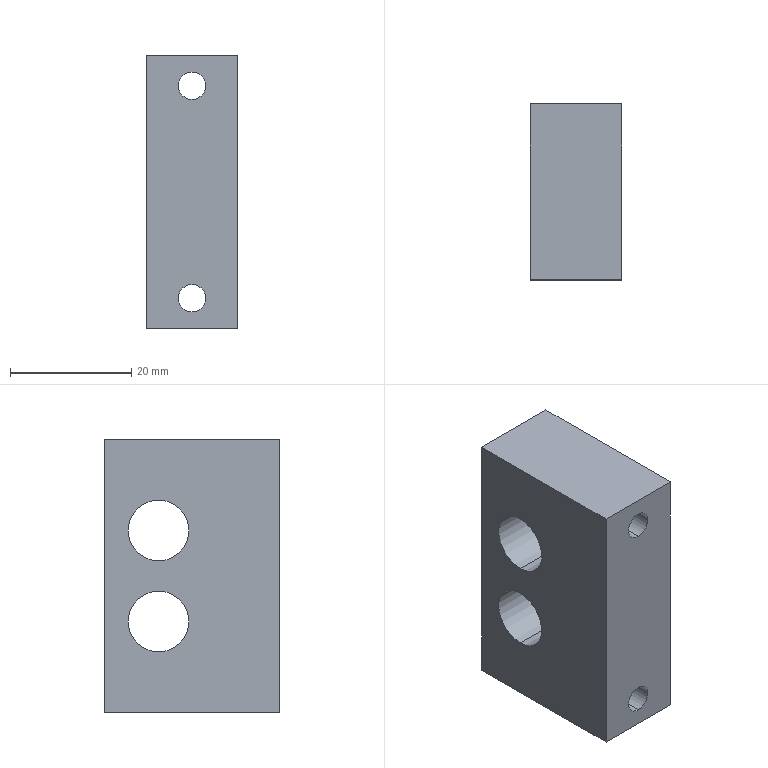Part | STEP file | 0246_218_Block | 1 solid | 14 faces | box 15 x 29 x 45 mm | volume 16296 mm3 | cylinder 8 | plane 6 | commonest cylinder face diameters 4.5 x4 10 x4
STEP:
#1=CARTESIAN_POINT('',(0.,0.,0.));
#2=DIRECTION('',(0.,0.,1.));
#3=DIRECTION('',(1.,0.,0.));
#4=AXIS2_PLACEMENT_3D('',#1,#2,#3);
#5=CARTESIAN_POINT('',(-7.5,0.,-15.25));
#6=VERTEX_POINT('',#5);
#7=CARTESIAN_POINT('',(-7.5,29.,-15.25));
#8=VERTEX_POINT('',#7);
#9=CARTESIAN_POINT('',(-7.5,29.,-15.25));
#10=DIRECTION('',(0.,1.,0.));
#11=VECTOR('',#10,1.);
#12=LINE('',#9,#11);
#13=CARTESIAN_POINT('',(-7.5,29.,-17.5));
#14=DIRECTION('',(0.,1.,0.));
#15=DIRECTION('',(0.,0.,1.));
#16=AXIS2_PLACEMENT_3D('',#13,#14,#15);
#17=CYLINDRICAL_SURFACE('',#16,2.25);
#18=CARTESIAN_POINT('',(6.283,0.));
#19=DIRECTION('',(0.,1.));
#20=VECTOR('',#19,1.);
#21=LINE('',#18,#20);
#22=(GEOMETRIC_REPRESENTATION_CONTEXT(2)PARAMETRIC_REPRESENTATION_CONTEXT()REPRESENTATION_CONTEXT('',''));
#23=DEFINITIONAL_REPRESENTATION('',(#21),#22);
#24=PCURVE('',#17,#23);
#25=CARTESIAN_POINT('',(-7.5,29.,-17.5));
#26=DIRECTION('',(0.,1.,0.));
#27=DIRECTION('',(0.,0.,1.));
#28=AXIS2_PLACEMENT_3D('',#25,#26,#27);
#29=CYLINDRICAL_SURFACE('',#28,2.25);
#30=CARTESIAN_POINT('',(0.,0.));
#31=DIRECTION('',(0.,1.));
#32=VECTOR('',#31,1.);
#33=LINE('',#30,#32);
#34=(GEOMETRIC_REPRESENTATION_CONTEXT(2)PARAMETRIC_REPRESENTATION_CONTEXT()REPRESENTATION_CONTEXT('',''));
#35=DEFINITIONAL_REPRESENTATION('',(#33),#34);
#36=PCURVE('',#29,#35);
#37=SURFACE_CURVE('',#12,(#24,#36),.PCURVE_S1.);
#38=EDGE_CURVE('',#6,#8,#37,.T.);
#39=ORIENTED_EDGE('',*,*,#38,.T.);
#40=CARTESIAN_POINT('',(-7.5,29.,-19.75));
#41=VERTEX_POINT('',#40);
#42=CARTESIAN_POINT('',(-7.5,29.,-17.5));
#43=DIRECTION('',(0.,1.,0.));
#44=DIRECTION('',(0.,0.,1.));
#45=AXIS2_PLACEMENT_3D('',#42,#43,#44);
#46=CIRCLE('',#45,2.25);
#47=CARTESIAN_POINT('',(0.,0.));
#48=DIRECTION('',(1.,0.));
#49=VECTOR('',#48,1.);
#50=LINE('',#47,#49);
#51=(GEOMETRIC_REPRESENTATION_CONTEXT(2)PARAMETRIC_REPRESENTATION_CONTEXT()REPRESENTATION_CONTEXT('',''));
#52=DEFINITIONAL_REPRESENTATION('',(#50),#51);
#53=PCURVE('',#17,#52);
#54=CARTESIAN_POINT('',(-15.,29.,22.5));
#55=DIRECTION('',(0.,1.,0.));
#56=DIRECTION('',(0.,0.,1.));
#57=AXIS2_PLACEMENT_3D('',#54,#55,#56);
#58=PLANE('',#57);
#59=CARTESIAN_POINT('',(-40.,7.5));
#60=DIRECTION('',(1.,0.));
#61=AXIS2_PLACEMENT_2D('',#59,#60);
#62=CIRCLE('',#61,2.25);
#63=(GEOMETRIC_REPRESENTATION_CONTEXT(2)PARAMETRIC_REPRESENTATION_CONTEXT()REPRESENTATION_CONTEXT('',''));
#64=DEFINITIONAL_REPRESENTATION('',(#62),#63);
#65=PCURVE('',#58,#64);
#66=SURFACE_CURVE('',#46,(#53,#65),.PCURVE_S1.);
#67=EDGE_CURVE('',#41,#8,#66,.T.);
#68=ORIENTED_EDGE('',*,*,#67,.F.);
#69=CARTESIAN_POINT('',(-7.5,0.,-19.75));
#70=VERTEX_POINT('',#69);
#71=CARTESIAN_POINT('',(-7.5,29.,-19.75));
#72=DIRECTION('',(0.,1.,0.));
#73=VECTOR('',#72,1.);
#74=LINE('',#71,#73);
#75=CARTESIAN_POINT('',(3.142,0.));
#76=DIRECTION('',(0.,1.));
#77=VECTOR('',#76,1.);
#78=LINE('',#75,#77);
#79=(GEOMETRIC_REPRESENTATION_CONTEXT(2)PARAMETRIC_REPRESENTATION_CONTEXT()REPRESENTATION_CONTEXT('',''));
#80=DEFINITIONAL_REPRESENTATION('',(#78),#79);
#81=PCURVE('',#17,#80);
#82=CARTESIAN_POINT('',(3.142,0.));
#83=DIRECTION('',(0.,1.));
#84=VECTOR('',#83,1.);
#85=LINE('',#82,#84);
#86=(GEOMETRIC_REPRESENTATION_CONTEXT(2)PARAMETRIC_REPRESENTATION_CONTEXT()REPRESENTATION_CONTEXT('',''));
#87=DEFINITIONAL_REPRESENTATION('',(#85),#86);
#88=PCURVE('',#29,#87);
#89=SURFACE_CURVE('',#74,(#81,#88),.PCURVE_S1.);
#90=EDGE_CURVE('',#70,#41,#89,.T.);
#91=ORIENTED_EDGE('',*,*,#90,.F.);
#92=CARTESIAN_POINT('',(-7.5,0.,-17.5));
#93=DIRECTION('',(0.,1.,0.));
#94=DIRECTION('',(0.,0.,1.));
#95=AXIS2_PLACEMENT_3D('',#92,#93,#94);
#96=CIRCLE('',#95,2.25);
#97=CARTESIAN_POINT('',(0.,-29.));
#98=DIRECTION('',(1.,0.));
#99=VECTOR('',#98,1.);
#100=LINE('',#97,#99);
#101=(GEOMETRIC_REPRESENTATION_CONTEXT(2)PARAMETRIC_REPRESENTATION_CONTEXT()REPRESENTATION_CONTEXT('',''));
#102=DEFINITIONAL_REPRESENTATION('',(#100),#101);
#103=PCURVE('',#17,#102);
#104=CARTESIAN_POINT('',(-15.,0.,22.5));
#105=DIRECTION('',(0.,-1.,0.));
#106=DIRECTION('',(0.,0.,-1.));
#107=AXIS2_PLACEMENT_3D('',#104,#105,#106);
#108=PLANE('',#107);
#109=CARTESIAN_POINT('',(37.75,7.5));
#110=CARTESIAN_POINT('',(37.75,11.397));
#111=CARTESIAN_POINT('',(41.125,9.449));
#112=CARTESIAN_POINT('',(44.5,7.5));
#113=CARTESIAN_POINT('',(41.125,5.551));
#114=CARTESIAN_POINT('',(37.75,3.603));
#115=CARTESIAN_POINT('',(37.75,7.5));
#116=(BOUNDED_CURVE()B_SPLINE_CURVE(2,(#109,#110,#111,#112,#113,#114,#115),.UNSPECIFIED.,.T.,.F.)B_SPLINE_CURVE_WITH_KNOTS((1,2,2,2,2,1),(-2.094,0.,2.094,4.189,6.283,8.378),.UNSPECIFIED.)CURVE()GEOMETRIC_REPRESENTATION_ITEM()RATIONAL_B_SPLINE_CURVE((1.,0.5,1.,0.5,1.,0.5,1.))REPRESENTATION_ITEM(''));
#117=(GEOMETRIC_REPRESENTATION_CONTEXT(2)PARAMETRIC_REPRESENTATION_CONTEXT()REPRESENTATION_CONTEXT('',''));
#118=DEFINITIONAL_REPRESENTATION('',(#116),#117);
#119=PCURVE('',#108,#118);
#120=SURFACE_CURVE('',#96,(#103,#119),.PCURVE_S1.);
#121=EDGE_CURVE('',#70,#6,#120,.T.);
#122=ORIENTED_EDGE('',*,*,#121,.T.);
#123=EDGE_LOOP('',(#39,#68,#91,#122));
#124=FACE_BOUND('',#123,.F.);
#125=ADVANCED_FACE('',(#124),#17,.F.);
#126=CARTESIAN_POINT('',(-7.5,0.,19.75));
#127=VERTEX_POINT('',#126);
#128=CARTESIAN_POINT('',(-7.5,29.,19.75));
#129=VERTEX_POINT('',#128);
#130=CARTESIAN_POINT('',(-7.5,29.,19.75));
#131=DIRECTION('',(0.,1.,0.));
#132=VECTOR('',#131,1.);
#133=LINE('',#130,#132);
#134=CARTESIAN_POINT('',(-7.5,29.,17.5));
#135=DIRECTION('',(0.,1.,0.));
#136=DIRECTION('',(0.,0.,1.));
#137=AXIS2_PLACEMENT_3D('',#134,#135,#136);
#138=CYLINDRICAL_SURFACE('',#137,2.25);
#139=CARTESIAN_POINT('',(6.283,0.));
#140=DIRECTION('',(0.,1.));
#141=VECTOR('',#140,1.);
#142=LINE('',#139,#141);
#143=(GEOMETRIC_REPRESENTATION_CONTEXT(2)PARAMETRIC_REPRESENTATION_CONTEXT()REPRESENTATION_CONTEXT('',''));
#144=DEFINITIONAL_REPRESENTATION('',(#142),#143);
#145=PCURVE('',#138,#144);
#146=CARTESIAN_POINT('',(-7.5,29.,17.5));
#147=DIRECTION('',(0.,1.,0.));
#148=DIRECTION('',(0.,0.,1.));
#149=AXIS2_PLACEMENT_3D('',#146,#147,#148);
#150=CYLINDRICAL_SURFACE('',#149,2.25);
#151=CARTESIAN_POINT('',(0.,0.));
#152=DIRECTION('',(0.,1.));
#153=VECTOR('',#152,1.);
#154=LINE('',#151,#153);
#155=(GEOMETRIC_REPRESENTATION_CONTEXT(2)PARAMETRIC_REPRESENTATION_CONTEXT()REPRESENTATION_CONTEXT('',''));
#156=DEFINITIONAL_REPRESENTATION('',(#154),#155);
#157=PCURVE('',#150,#156);
#158=SURFACE_CURVE('',#133,(#145,#157),.PCURVE_S1.);
#159=EDGE_CURVE('',#127,#129,#158,.T.);
#160=ORIENTED_EDGE('',*,*,#159,.T.);
#161=CARTESIAN_POINT('',(-7.5,29.,15.25));
#162=VERTEX_POINT('',#161);
#163=CARTESIAN_POINT('',(-7.5,29.,17.5));
#164=DIRECTION('',(0.,1.,0.));
#165=DIRECTION('',(0.,0.,1.));
#166=AXIS2_PLACEMENT_3D('',#163,#164,#165);
#167=CIRCLE('',#166,2.25);
#168=CARTESIAN_POINT('',(0.,0.));
#169=DIRECTION('',(1.,0.));
#170=VECTOR('',#169,1.);
#171=LINE('',#168,#170);
#172=(GEOMETRIC_REPRESENTATION_CONTEXT(2)PARAMETRIC_REPRESENTATION_CONTEXT()REPRESENTATION_CONTEXT('',''));
#173=DEFINITIONAL_REPRESENTATION('',(#171),#172);
#174=PCURVE('',#138,#173);
#175=CARTESIAN_POINT('',(-5.,7.5));
#176=DIRECTION('',(1.,0.));
#177=AXIS2_PLACEMENT_2D('',#175,#176);
#178=CIRCLE('',#177,2.25);
#179=(GEOMETRIC_REPRESENTATION_CONTEXT(2)PARAMETRIC_REPRESENTATION_CONTEXT()REPRESENTATION_CONTEXT('',''));
#180=DEFINITIONAL_REPRESENTATION('',(#178),#179);
#181=PCURVE('',#58,#180);
#182=SURFACE_CURVE('',#167,(#174,#181),.PCURVE_S1.);
#183=EDGE_CURVE('',#162,#129,#182,.T.);
#184=ORIENTED_EDGE('',*,*,#183,.F.);
#185=CARTESIAN_POINT('',(-7.5,0.,15.25));
#186=VERTEX_POINT('',#185);
#187=CARTESIAN_POINT('',(-7.5,29.,15.25));
#188=DIRECTION('',(0.,1.,0.));
#189=VECTOR('',#188,1.);
#190=LINE('',#187,#189);
#191=CARTESIAN_POINT('',(3.142,0.));
#192=DIRECTION('',(0.,1.));
#193=VECTOR('',#192,1.);
#194=LINE('',#191,#193);
#195=(GEOMETRIC_REPRESENTATION_CONTEXT(2)PARAMETRIC_REPRESENTATION_CONTEXT()REPRESENTATION_CONTEXT('',''));
#196=DEFINITIONAL_REPRESENTATION('',(#194),#195);
#197=PCURVE('',#138,#196);
#198=CARTESIAN_POINT('',(3.142,0.));
#199=DIRECTION('',(0.,1.));
#200=VECTOR('',#199,1.);
#201=LINE('',#198,#200);
#202=(GEOMETRIC_REPRESENTATION_CONTEXT(2)PARAMETRIC_REPRESENTATION_CONTEXT()REPRESENTATION_CONTEXT('',''));
#203=DEFINITIONAL_REPRESENTATION('',(#201),#202);
#204=PCURVE('',#150,#203);
#205=SURFACE_CURVE('',#190,(#197,#204),.PCURVE_S1.);
#206=EDGE_CURVE('',#186,#162,#205,.T.);
#207=ORIENTED_EDGE('',*,*,#206,.F.);
#208=CARTESIAN_POINT('',(-7.5,0.,17.5));
#209=DIRECTION('',(0.,1.,0.));
#210=DIRECTION('',(0.,0.,1.));
#211=AXIS2_PLACEMENT_3D('',#208,#209,#210);
#212=CIRCLE('',#211,2.25);
#213=CARTESIAN_POINT('',(0.,-29.));
#214=DIRECTION('',(1.,0.));
#215=VECTOR('',#214,1.);
#216=LINE('',#213,#215);
#217=(GEOMETRIC_REPRESENTATION_CONTEXT(2)PARAMETRIC_REPRESENTATION_CONTEXT()REPRESENTATION_CONTEXT('',''));
#218=DEFINITIONAL_REPRESENTATION('',(#216),#217);
#219=PCURVE('',#138,#218);
#220=CARTESIAN_POINT('',(2.75,7.5));
#221=CARTESIAN_POINT('',(2.75,11.397));
#222=CARTESIAN_POINT('',(6.125,9.449));
#223=CARTESIAN_POINT('',(9.5,7.5));
#224=CARTESIAN_POINT('',(6.125,5.551));
#225=CARTESIAN_POINT('',(2.75,3.603));
#226=CARTESIAN_POINT('',(2.75,7.5));
#227=(BOUNDED_CURVE()B_SPLINE_CURVE(2,(#220,#221,#222,#223,#224,#225,#226),.UNSPECIFIED.,.T.,.F.)B_SPLINE_CURVE_WITH_KNOTS((1,2,2,2,2,1),(-2.094,0.,2.094,4.189,6.283,8.378),.UNSPECIFIED.)CURVE()GEOMETRIC_REPRESENTATION_ITEM()RATIONAL_B_SPLINE_CURVE((1.,0.5,1.,0.5,1.,0.5,1.))REPRESENTATION_ITEM(''));
#228=(GEOMETRIC_REPRESENTATION_CONTEXT(2)PARAMETRIC_REPRESENTATION_CONTEXT()REPRESENTATION_CONTEXT('',''));
#229=DEFINITIONAL_REPRESENTATION('',(#227),#228);
#230=PCURVE('',#108,#229);
#231=SURFACE_CURVE('',#212,(#219,#230),.PCURVE_S1.);
#232=EDGE_CURVE('',#186,#127,#231,.T.);
#233=ORIENTED_EDGE('',*,*,#232,.T.);
#234=EDGE_LOOP('',(#160,#184,#207,#233));
#235=FACE_BOUND('',#234,.F.);
#236=ADVANCED_FACE('',(#235),#138,.F.);
#237=CARTESIAN_POINT('',(0.,20.,-2.5));
#238=VERTEX_POINT('',#237);
#239=CARTESIAN_POINT('',(-15.,20.,-2.5));
#240=VERTEX_POINT('',#239);
#241=CARTESIAN_POINT('',(-15.,20.,-2.5));
#242=DIRECTION('',(-1.,0.,0.));
#243=VECTOR('',#242,1.);
#244=LINE('',#241,#243);
#245=CARTESIAN_POINT('',(-15.,20.,-7.5));
#246=DIRECTION('',(-1.,0.,0.));
#247=DIRECTION('',(0.,0.,1.));
#248=AXIS2_PLACEMENT_3D('',#245,#246,#247);
#249=CYLINDRICAL_SURFACE('',#248,5.);
#250=CARTESIAN_POINT('',(6.283,0.));
#251=DIRECTION('',(0.,1.));
#252=VECTOR('',#251,1.);
#253=LINE('',#250,#252);
#254=(GEOMETRIC_REPRESENTATION_CONTEXT(2)PARAMETRIC_REPRESENTATION_CONTEXT()REPRESENTATION_CONTEXT('',''));
#255=DEFINITIONAL_REPRESENTATION('',(#253),#254);
#256=PCURVE('',#249,#255);
#257=CARTESIAN_POINT('',(-15.,20.,-7.5));
#258=DIRECTION('',(-1.,0.,0.));
#259=DIRECTION('',(0.,0.,1.));
#260=AXIS2_PLACEMENT_3D('',#257,#258,#259);
#261=CYLINDRICAL_SURFACE('',#260,5.);
#262=CARTESIAN_POINT('',(0.,0.));
#263=DIRECTION('',(0.,1.));
#264=VECTOR('',#263,1.);
#265=LINE('',#262,#264);
#266=(GEOMETRIC_REPRESENTATION_CONTEXT(2)PARAMETRIC_REPRESENTATION_CONTEXT()REPRESENTATION_CONTEXT('',''));
#267=DEFINITIONAL_REPRESENTATION('',(#265),#266);
#268=PCURVE('',#261,#267);
#269=SURFACE_CURVE('',#244,(#256,#268),.PCURVE_S1.);
#270=EDGE_CURVE('',#238,#240,#269,.T.);
#271=ORIENTED_EDGE('',*,*,#270,.T.);
#272=CARTESIAN_POINT('',(-15.,20.,-12.5));
#273=VERTEX_POINT('',#272);
#274=CARTESIAN_POINT('',(-15.,20.,-7.5));
#275=DIRECTION('',(-1.,0.,0.));
#276=DIRECTION('',(0.,0.,1.));
#277=AXIS2_PLACEMENT_3D('',#274,#275,#276);
#278=CIRCLE('',#277,5.);
#279=CARTESIAN_POINT('',(0.,0.));
#280=DIRECTION('',(1.,0.));
#281=VECTOR('',#280,1.);
#282=LINE('',#279,#281);
#283=(GEOMETRIC_REPRESENTATION_CONTEXT(2)PARAMETRIC_REPRESENTATION_CONTEXT()REPRESENTATION_CONTEXT('',''));
#284=DEFINITIONAL_REPRESENTATION('',(#282),#283);
#285=PCURVE('',#249,#284);
#286=CARTESIAN_POINT('',(-15.,0.,22.5));
#287=DIRECTION('',(1.,0.,0.));
#288=DIRECTION('',(0.,0.,-1.));
#289=AXIS2_PLACEMENT_3D('',#286,#287,#288);
#290=PLANE('',#289);
#291=CARTESIAN_POINT('',(25.,20.));
#292=CARTESIAN_POINT('',(25.,28.66));
#293=CARTESIAN_POINT('',(32.5,24.33));
#294=CARTESIAN_POINT('',(40.,20.));
#295=CARTESIAN_POINT('',(32.5,15.67));
#296=CARTESIAN_POINT('',(25.,11.34));
#297=CARTESIAN_POINT('',(25.,20.));
#298=(BOUNDED_CURVE()B_SPLINE_CURVE(2,(#291,#292,#293,#294,#295,#296,#297),.UNSPECIFIED.,.T.,.F.)B_SPLINE_CURVE_WITH_KNOTS((1,2,2,2,2,1),(-2.094,0.,2.094,4.189,6.283,8.378),.UNSPECIFIED.)CURVE()GEOMETRIC_REPRESENTATION_ITEM()RATIONAL_B_SPLINE_CURVE((1.,0.5,1.,0.5,1.,0.5,1.))REPRESENTATION_ITEM(''));
#299=(GEOMETRIC_REPRESENTATION_CONTEXT(2)PARAMETRIC_REPRESENTATION_CONTEXT()REPRESENTATION_CONTEXT('',''));
#300=DEFINITIONAL_REPRESENTATION('',(#298),#299);
#301=PCURVE('',#290,#300);
#302=SURFACE_CURVE('',#278,(#285,#301),.PCURVE_S1.);
#303=EDGE_CURVE('',#273,#240,#302,.T.);
#304=ORIENTED_EDGE('',*,*,#303,.F.);
#305=CARTESIAN_POINT('',(0.,20.,-12.5));
#306=VERTEX_POINT('',#305);
#307=CARTESIAN_POINT('',(-15.,20.,-12.5));
#308=DIRECTION('',(-1.,0.,0.));
#309=VECTOR('',#308,1.);
#310=LINE('',#307,#309);
#311=CARTESIAN_POINT('',(3.142,0.));
#312=DIRECTION('',(0.,1.));
#313=VECTOR('',#312,1.);
#314=LINE('',#311,#313);
#315=(GEOMETRIC_REPRESENTATION_CONTEXT(2)PARAMETRIC_REPRESENTATION_CONTEXT()REPRESENTATION_CONTEXT('',''));
#316=DEFINITIONAL_REPRESENTATION('',(#314),#315);
#317=PCURVE('',#249,#316);
#318=CARTESIAN_POINT('',(3.142,0.));
#319=DIRECTION('',(0.,1.));
#320=VECTOR('',#319,1.);
#321=LINE('',#318,#320);
#322=(GEOMETRIC_REPRESENTATION_CONTEXT(2)PARAMETRIC_REPRESENTATION_CONTEXT()REPRESENTATION_CONTEXT('',''));
#323=DEFINITIONAL_REPRESENTATION('',(#321),#322);
#324=PCURVE('',#261,#323);
#325=SURFACE_CURVE('',#310,(#317,#324),.PCURVE_S1.);
#326=EDGE_CURVE('',#306,#273,#325,.T.);
#327=ORIENTED_EDGE('',*,*,#326,.F.);
#328=CARTESIAN_POINT('',(0.,20.,-7.5));
#329=DIRECTION('',(-1.,0.,0.));
#330=DIRECTION('',(0.,0.,1.));
#331=AXIS2_PLACEMENT_3D('',#328,#329,#330);
#332=CIRCLE('',#331,5.);
#333=CARTESIAN_POINT('',(0.,-15.));
#334=DIRECTION('',(1.,0.));
#335=VECTOR('',#334,1.);
#336=LINE('',#333,#335);
#337=(GEOMETRIC_REPRESENTATION_CONTEXT(2)PARAMETRIC_REPRESENTATION_CONTEXT()REPRESENTATION_CONTEXT('',''));
#338=DEFINITIONAL_REPRESENTATION('',(#336),#337);
#339=PCURVE('',#249,#338);
#340=CARTESIAN_POINT('',(0.,0.,22.5));
#341=DIRECTION('',(1.,0.,0.));
#342=DIRECTION('',(0.,0.,-1.));
#343=AXIS2_PLACEMENT_3D('',#340,#341,#342);
#344=PLANE('',#343);
#345=CARTESIAN_POINT('',(25.,20.));
#346=CARTESIAN_POINT('',(25.,28.66));
#347=CARTESIAN_POINT('',(32.5,24.33));
#348=CARTESIAN_POINT('',(40.,20.));
#349=CARTESIAN_POINT('',(32.5,15.67));
#350=CARTESIAN_POINT('',(25.,11.34));
#351=CARTESIAN_POINT('',(25.,20.));
#352=(BOUNDED_CURVE()B_SPLINE_CURVE(2,(#345,#346,#347,#348,#349,#350,#351),.UNSPECIFIED.,.T.,.F.)B_SPLINE_CURVE_WITH_KNOTS((1,2,2,2,2,1),(-2.094,0.,2.094,4.189,6.283,8.378),.UNSPECIFIED.)CURVE()GEOMETRIC_REPRESENTATION_ITEM()RATIONAL_B_SPLINE_CURVE((1.,0.5,1.,0.5,1.,0.5,1.))REPRESENTATION_ITEM(''));
#353=(GEOMETRIC_REPRESENTATION_CONTEXT(2)PARAMETRIC_REPRESENTATION_CONTEXT()REPRESENTATION_CONTEXT('',''));
#354=DEFINITIONAL_REPRESENTATION('',(#352),#353);
#355=PCURVE('',#344,#354);
#356=SURFACE_CURVE('',#332,(#339,#355),.PCURVE_S1.);
#357=EDGE_CURVE('',#306,#238,#356,.T.);
#358=ORIENTED_EDGE('',*,*,#357,.T.);
#359=EDGE_LOOP('',(#271,#304,#327,#358));
#360=FACE_BOUND('',#359,.F.);
#361=ADVANCED_FACE('',(#360),#249,.F.);
#362=CARTESIAN_POINT('',(0.,20.,12.5));
#363=VERTEX_POINT('',#362);
#364=CARTESIAN_POINT('',(-15.,20.,12.5));
#365=VERTEX_POINT('',#364);
#366=CARTESIAN_POINT('',(-15.,20.,12.5));
#367=DIRECTION('',(-1.,0.,0.));
#368=VECTOR('',#367,1.);
#369=LINE('',#366,#368);
#370=CARTESIAN_POINT('',(-15.,20.,7.5));
#371=DIRECTION('',(-1.,0.,0.));
#372=DIRECTION('',(0.,0.,1.));
#373=AXIS2_PLACEMENT_3D('',#370,#371,#372);
#374=CYLINDRICAL_SURFACE('',#373,5.);
#375=CARTESIAN_POINT('',(6.283,0.));
#376=DIRECTION('',(0.,1.));
#377=VECTOR('',#376,1.);
#378=LINE('',#375,#377);
#379=(GEOMETRIC_REPRESENTATION_CONTEXT(2)PARAMETRIC_REPRESENTATION_CONTEXT()REPRESENTATION_CONTEXT('',''));
#380=DEFINITIONAL_REPRESENTATION('',(#378),#379);
#381=PCURVE('',#374,#380);
#382=CARTESIAN_POINT('',(-15.,20.,7.5));
#383=DIRECTION('',(-1.,0.,0.));
#384=DIRECTION('',(0.,0.,1.));
#385=AXIS2_PLACEMENT_3D('',#382,#383,#384);
#386=CYLINDRICAL_SURFACE('',#385,5.);
#387=CARTESIAN_POINT('',(0.,0.));
#388=DIRECTION('',(0.,1.));
#389=VECTOR('',#388,1.);
#390=LINE('',#387,#389);
#391=(GEOMETRIC_REPRESENTATION_CONTEXT(2)PARAMETRIC_REPRESENTATION_CONTEXT()REPRESENTATION_CONTEXT('',''));
#392=DEFINITIONAL_REPRESENTATION('',(#390),#391);
#393=PCURVE('',#386,#392);
#394=SURFACE_CURVE('',#369,(#381,#393),.PCURVE_S1.);
#395=EDGE_CURVE('',#363,#365,#394,.T.);
#396=ORIENTED_EDGE('',*,*,#395,.T.);
#397=CARTESIAN_POINT('',(-15.,20.,2.5));
#398=VERTEX_POINT('',#397);
#399=CARTESIAN_POINT('',(-15.,20.,7.5));
#400=DIRECTION('',(-1.,0.,0.));
#401=DIRECTION('',(0.,0.,1.));
#402=AXIS2_PLACEMENT_3D('',#399,#400,#401);
#403=CIRCLE('',#402,5.);
#404=CARTESIAN_POINT('',(0.,0.));
#405=DIRECTION('',(1.,0.));
#406=VECTOR('',#405,1.);
#407=LINE('',#404,#406);
#408=(GEOMETRIC_REPRESENTATION_CONTEXT(2)PARAMETRIC_REPRESENTATION_CONTEXT()REPRESENTATION_CONTEXT('',''));
#409=DEFINITIONAL_REPRESENTATION('',(#407),#408);
#410=PCURVE('',#374,#409);
#411=CARTESIAN_POINT('',(10.,20.));
#412=CARTESIAN_POINT('',(10.,28.66));
#413=CARTESIAN_POINT('',(17.5,24.33));
#414=CARTESIAN_POINT('',(25.,20.));
#415=CARTESIAN_POINT('',(17.5,15.67));
#416=CARTESIAN_POINT('',(10.,11.34));
#417=CARTESIAN_POINT('',(10.,20.));
#418=(BOUNDED_CURVE()B_SPLINE_CURVE(2,(#411,#412,#413,#414,#415,#416,#417),.UNSPECIFIED.,.T.,.F.)B_SPLINE_CURVE_WITH_KNOTS((1,2,2,2,2,1),(-2.094,0.,2.094,4.189,6.283,8.378),.UNSPECIFIED.)CURVE()GEOMETRIC_REPRESENTATION_ITEM()RATIONAL_B_SPLINE_CURVE((1.,0.5,1.,0.5,1.,0.5,1.))REPRESENTATION_ITEM(''));
#419=(GEOMETRIC_REPRESENTATION_CONTEXT(2)PARAMETRIC_REPRESENTATION_CONTEXT()REPRESENTATION_CONTEXT('',''));
#420=DEFINITIONAL_REPRESENTATION('',(#418),#419);
#421=PCURVE('',#290,#420);
#422=SURFACE_CURVE('',#403,(#410,#421),.PCURVE_S1.);
#423=EDGE_CURVE('',#398,#365,#422,.T.);
#424=ORIENTED_EDGE('',*,*,#423,.F.);
#425=CARTESIAN_POINT('',(0.,20.,2.5));
#426=VERTEX_POINT('',#425);
#427=CARTESIAN_POINT('',(-15.,20.,2.5));
#428=DIRECTION('',(-1.,0.,0.));
#429=VECTOR('',#428,1.);
#430=LINE('',#427,#429);
#431=CARTESIAN_POINT('',(3.142,0.));
#432=DIRECTION('',(0.,1.));
#433=VECTOR('',#432,1.);
#434=LINE('',#431,#433);
#435=(GEOMETRIC_REPRESENTATION_CONTEXT(2)PARAMETRIC_REPRESENTATION_CONTEXT()REPRESENTATION_CONTEXT('',''));
#436=DEFINITIONAL_REPRESENTATION('',(#434),#435);
#437=PCURVE('',#374,#436);
#438=CARTESIAN_POINT('',(3.142,0.));
#439=DIRECTION('',(0.,1.));
#440=VECTOR('',#439,1.);
#441=LINE('',#438,#440);
#442=(GEOMETRIC_REPRESENTATION_CONTEXT(2)PARAMETRIC_REPRESENTATION_CONTEXT()REPRESENTATION_CONTEXT('',''));
#443=DEFINITIONAL_REPRESENTATION('',(#441),#442);
#444=PCURVE('',#386,#443);
#445=SURFACE_CURVE('',#430,(#437,#444),.PCURVE_S1.);
#446=EDGE_CURVE('',#426,#398,#445,.T.);
#447=ORIENTED_EDGE('',*,*,#446,.F.);
#448=CARTESIAN_POINT('',(0.,20.,7.5));
#449=DIRECTION('',(-1.,0.,0.));
#450=DIRECTION('',(0.,0.,1.));
#451=AXIS2_PLACEMENT_3D('',#448,#449,#450);
#452=CIRCLE('',#451,5.);
#453=CARTESIAN_POINT('',(0.,-15.));
#454=DIRECTION('',(1.,0.));
#455=VECTOR('',#454,1.);
#456=LINE('',#453,#455);
#457=(GEOMETRIC_REPRESENTATION_CONTEXT(2)PARAMETRIC_REPRESENTATION_CONTEXT()REPRESENTATION_CONTEXT('',''));
#458=DEFINITIONAL_REPRESENTATION('',(#456),#457);
#459=PCURVE('',#374,#458);
#460=CARTESIAN_POINT('',(10.,20.));
#461=CARTESIAN_POINT('',(10.,28.66));
#462=CARTESIAN_POINT('',(17.5,24.33));
#463=CARTESIAN_POINT('',(25.,20.));
#464=CARTESIAN_POINT('',(17.5,15.67));
#465=CARTESIAN_POINT('',(10.,11.34));
#466=CARTESIAN_POINT('',(10.,20.));
#467=(BOUNDED_CURVE()B_SPLINE_CURVE(2,(#460,#461,#462,#463,#464,#465,#466),.UNSPECIFIED.,.T.,.F.)B_SPLINE_CURVE_WITH_KNOTS((1,2,2,2,2,1),(-2.094,0.,2.094,4.189,6.283,8.378),.UNSPECIFIED.)CURVE()GEOMETRIC_REPRESENTATION_ITEM()RATIONAL_B_SPLINE_CURVE((1.,0.5,1.,0.5,1.,0.5,1.))REPRESENTATION_ITEM(''));
#468=(GEOMETRIC_REPRESENTATION_CONTEXT(2)PARAMETRIC_REPRESENTATION_CONTEXT()REPRESENTATION_CONTEXT('',''));
#469=DEFINITIONAL_REPRESENTATION('',(#467),#468);
#470=PCURVE('',#344,#469);
#471=SURFACE_CURVE('',#452,(#459,#470),.PCURVE_S1.);
#472=EDGE_CURVE('',#426,#363,#471,.T.);
#473=ORIENTED_EDGE('',*,*,#472,.T.);
#474=EDGE_LOOP('',(#396,#424,#447,#473));
#475=FACE_BOUND('',#474,.F.);
#476=ADVANCED_FACE('',(#475),#374,.F.);
#477=CARTESIAN_POINT('',(0.,29.,22.5));
#478=VERTEX_POINT('',#477);
#479=CARTESIAN_POINT('',(0.,0.,22.5));
#480=VERTEX_POINT('',#479);
#481=CARTESIAN_POINT('',(0.,29.,22.5));
#482=DIRECTION('',(0.,-1.,0.));
#483=VECTOR('',#482,1.);
#484=LINE('',#481,#483);
#485=CARTESIAN_POINT('',(-15.,29.,22.5));
#486=DIRECTION('',(0.,0.,1.));
#487=DIRECTION('',(0.,-1.,0.));
#488=AXIS2_PLACEMENT_3D('',#485,#486,#487);
#489=PLANE('',#488);
#490=CARTESIAN_POINT('',(0.,15.));
#491=DIRECTION('',(1.,0.));
#492=VECTOR('',#491,1.);
#493=LINE('',#490,#492);
#494=(GEOMETRIC_REPRESENTATION_CONTEXT(2)PARAMETRIC_REPRESENTATION_CONTEXT()REPRESENTATION_CONTEXT('',''));
#495=DEFINITIONAL_REPRESENTATION('',(#493),#494);
#496=PCURVE('',#489,#495);
#497=CARTESIAN_POINT('',(0.,29.));
#498=DIRECTION('',(0.,-1.));
#499=VECTOR('',#498,1.);
#500=LINE('',#497,#499);
#501=(GEOMETRIC_REPRESENTATION_CONTEXT(2)PARAMETRIC_REPRESENTATION_CONTEXT()REPRESENTATION_CONTEXT('',''));
#502=DEFINITIONAL_REPRESENTATION('',(#500),#501);
#503=PCURVE('',#344,#502);
#504=SURFACE_CURVE('',#484,(#496,#503),.PCURVE_S1.);
#505=EDGE_CURVE('',#478,#480,#504,.T.);
#506=ORIENTED_EDGE('',*,*,#505,.F.);
#507=CARTESIAN_POINT('',(-15.,29.,22.5));
#508=VERTEX_POINT('',#507);
#509=CARTESIAN_POINT('',(-15.,29.,22.5));
#510=DIRECTION('',(1.,0.,0.));
#511=VECTOR('',#510,1.);
#512=LINE('',#509,#511);
#513=CARTESIAN_POINT('',(0.,0.));
#514=DIRECTION('',(0.,1.));
#515=VECTOR('',#514,1.);
#516=LINE('',#513,#515);
#517=(GEOMETRIC_REPRESENTATION_CONTEXT(2)PARAMETRIC_REPRESENTATION_CONTEXT()REPRESENTATION_CONTEXT('',''));
#518=DEFINITIONAL_REPRESENTATION('',(#516),#517);
#519=PCURVE('',#489,#518);
#520=CARTESIAN_POINT('',(0.,0.));
#521=DIRECTION('',(0.,1.));
#522=VECTOR('',#521,1.);
#523=LINE('',#520,#522);
#524=(GEOMETRIC_REPRESENTATION_CONTEXT(2)PARAMETRIC_REPRESENTATION_CONTEXT()REPRESENTATION_CONTEXT('',''));
#525=DEFINITIONAL_REPRESENTATION('',(#523),#524);
#526=PCURVE('',#58,#525);
#527=SURFACE_CURVE('',#512,(#519,#526),.PCURVE_S1.);
#528=EDGE_CURVE('',#508,#478,#527,.T.);
#529=ORIENTED_EDGE('',*,*,#528,.F.);
#530=CARTESIAN_POINT('',(-15.,0.,22.5));
#531=VERTEX_POINT('',#530);
#532=CARTESIAN_POINT('',(-15.,29.,22.5));
#533=DIRECTION('',(0.,-1.,0.));
#534=VECTOR('',#533,1.);
#535=LINE('',#532,#534);
#536=CARTESIAN_POINT('',(0.,0.));
#537=DIRECTION('',(1.,0.));
#538=VECTOR('',#537,1.);
#539=LINE('',#536,#538);
#540=(GEOMETRIC_REPRESENTATION_CONTEXT(2)PARAMETRIC_REPRESENTATION_CONTEXT()REPRESENTATION_CONTEXT('',''));
#541=DEFINITIONAL_REPRESENTATION('',(#539),#540);
#542=PCURVE('',#489,#541);
#543=CARTESIAN_POINT('',(0.,29.));
#544=DIRECTION('',(0.,-1.));
#545=VECTOR('',#544,1.);
#546=LINE('',#543,#545);
#547=(GEOMETRIC_REPRESENTATION_CONTEXT(2)PARAMETRIC_REPRESENTATION_CONTEXT()REPRESENTATION_CONTEXT('',''));
#548=DEFINITIONAL_REPRESENTATION('',(#546),#547);
#549=PCURVE('',#290,#548);
#550=SURFACE_CURVE('',#535,(#542,#549),.PCURVE_S1.);
#551=EDGE_CURVE('',#508,#531,#550,.T.);
#552=ORIENTED_EDGE('',*,*,#551,.T.);
#553=CARTESIAN_POINT('',(-15.,0.,22.5));
#554=DIRECTION('',(1.,0.,0.));
#555=VECTOR('',#554,1.);
#556=LINE('',#553,#555);
#557=CARTESIAN_POINT('',(29.,0.));
#558=DIRECTION('',(0.,1.));
#559=VECTOR('',#558,1.);
#560=LINE('',#557,#559);
#561=(GEOMETRIC_REPRESENTATION_CONTEXT(2)PARAMETRIC_REPRESENTATION_CONTEXT()REPRESENTATION_CONTEXT('',''));
#562=DEFINITIONAL_REPRESENTATION('',(#560),#561);
#563=PCURVE('',#489,#562);
#564=CARTESIAN_POINT('',(0.,0.));
#565=DIRECTION('',(0.,1.));
#566=VECTOR('',#565,1.);
#567=LINE('',#564,#566);
#568=(GEOMETRIC_REPRESENTATION_CONTEXT(2)PARAMETRIC_REPRESENTATION_CONTEXT()REPRESENTATION_CONTEXT('',''));
#569=DEFINITIONAL_REPRESENTATION('',(#567),#568);
#570=PCURVE('',#108,#569);
#571=SURFACE_CURVE('',#556,(#563,#570),.PCURVE_S1.);
#572=EDGE_CURVE('',#531,#480,#571,.T.);
#573=ORIENTED_EDGE('',*,*,#572,.T.);
#574=EDGE_LOOP('',(#506,#529,#552,#573));
#575=FACE_BOUND('',#574,.T.);
#576=ADVANCED_FACE('',(#575),#489,.T.);
#577=CARTESIAN_POINT('',(-7.5,29.,-17.5));
#578=DIRECTION('',(0.,1.,0.));
#579=DIRECTION('',(0.,0.,1.));
#580=AXIS2_PLACEMENT_3D('',#577,#578,#579);
#581=CIRCLE('',#580,2.25);
#582=CARTESIAN_POINT('',(-40.,7.5));
#583=DIRECTION('',(1.,0.));
#584=AXIS2_PLACEMENT_2D('',#582,#583);
#585=CIRCLE('',#584,2.25);
#586=(GEOMETRIC_REPRESENTATION_CONTEXT(2)PARAMETRIC_REPRESENTATION_CONTEXT()REPRESENTATION_CONTEXT('',''));
#587=DEFINITIONAL_REPRESENTATION('',(#585),#586);
#588=PCURVE('',#58,#587);
#589=CARTESIAN_POINT('',(0.,0.));
#590=DIRECTION('',(1.,0.));
#591=VECTOR('',#590,1.);
#592=LINE('',#589,#591);
#593=(GEOMETRIC_REPRESENTATION_CONTEXT(2)PARAMETRIC_REPRESENTATION_CONTEXT()REPRESENTATION_CONTEXT('',''));
#594=DEFINITIONAL_REPRESENTATION('',(#592),#593);
#595=PCURVE('',#29,#594);
#596=SURFACE_CURVE('',#581,(#588,#595),.PCURVE_S1.);
#597=EDGE_CURVE('',#8,#41,#596,.T.);
#598=ORIENTED_EDGE('',*,*,#597,.F.);
#599=ORIENTED_EDGE('',*,*,#67,.F.);
#600=EDGE_LOOP('',(#598,#599));
#601=FACE_BOUND('',#600,.T.);
#602=CARTESIAN_POINT('',(-7.5,29.,17.5));
#603=DIRECTION('',(0.,1.,0.));
#604=DIRECTION('',(0.,0.,1.));
#605=AXIS2_PLACEMENT_3D('',#602,#603,#604);
#606=CIRCLE('',#605,2.25);
#607=CARTESIAN_POINT('',(-5.,7.5));
#608=DIRECTION('',(1.,0.));
#609=AXIS2_PLACEMENT_2D('',#607,#608);
#610=CIRCLE('',#609,2.25);
#611=(GEOMETRIC_REPRESENTATION_CONTEXT(2)PARAMETRIC_REPRESENTATION_CONTEXT()REPRESENTATION_CONTEXT('',''));
#612=DEFINITIONAL_REPRESENTATION('',(#610),#611);
#613=PCURVE('',#58,#612);
#614=CARTESIAN_POINT('',(0.,0.));
#615=DIRECTION('',(1.,0.));
#616=VECTOR('',#615,1.);
#617=LINE('',#614,#616);
#618=(GEOMETRIC_REPRESENTATION_CONTEXT(2)PARAMETRIC_REPRESENTATION_CONTEXT()REPRESENTATION_CONTEXT('',''));
#619=DEFINITIONAL_REPRESENTATION('',(#617),#618);
#620=PCURVE('',#150,#619);
#621=SURFACE_CURVE('',#606,(#613,#620),.PCURVE_S1.);
#622=EDGE_CURVE('',#129,#162,#621,.T.);
#623=ORIENTED_EDGE('',*,*,#622,.F.);
#624=ORIENTED_EDGE('',*,*,#183,.F.);
#625=EDGE_LOOP('',(#623,#624));
#626=FACE_BOUND('',#625,.T.);
#627=CARTESIAN_POINT('',(0.,29.,-22.5));
#628=VERTEX_POINT('',#627);
#629=CARTESIAN_POINT('',(0.,29.,22.5));
#630=DIRECTION('',(0.,0.,1.));
#631=VECTOR('',#630,1.);
#632=LINE('',#629,#631);
#633=CARTESIAN_POINT('',(0.,15.));
#634=DIRECTION('',(1.,0.));
#635=VECTOR('',#634,1.);
#636=LINE('',#633,#635);
#637=(GEOMETRIC_REPRESENTATION_CONTEXT(2)PARAMETRIC_REPRESENTATION_CONTEXT()REPRESENTATION_CONTEXT('',''));
#638=DEFINITIONAL_REPRESENTATION('',(#636),#637);
#639=PCURVE('',#58,#638);
#640=CARTESIAN_POINT('',(0.,29.));
#641=DIRECTION('',(-1.,0.));
#642=VECTOR('',#641,1.);
#643=LINE('',#640,#642);
#644=(GEOMETRIC_REPRESENTATION_CONTEXT(2)PARAMETRIC_REPRESENTATION_CONTEXT()REPRESENTATION_CONTEXT('',''));
#645=DEFINITIONAL_REPRESENTATION('',(#643),#644);
#646=PCURVE('',#344,#645);
#647=SURFACE_CURVE('',#632,(#639,#646),.PCURVE_S1.);
#648=EDGE_CURVE('',#628,#478,#647,.T.);
#649=ORIENTED_EDGE('',*,*,#648,.F.);
#650=CARTESIAN_POINT('',(-15.,29.,-22.5));
#651=VERTEX_POINT('',#650);
#652=CARTESIAN_POINT('',(-15.,29.,-22.5));
#653=DIRECTION('',(1.,0.,0.));
#654=VECTOR('',#653,1.);
#655=LINE('',#652,#654);
#656=CARTESIAN_POINT('',(-45.,0.));
#657=DIRECTION('',(0.,1.));
#658=VECTOR('',#657,1.);
#659=LINE('',#656,#658);
#660=(GEOMETRIC_REPRESENTATION_CONTEXT(2)PARAMETRIC_REPRESENTATION_CONTEXT()REPRESENTATION_CONTEXT('',''));
#661=DEFINITIONAL_REPRESENTATION('',(#659),#660);
#662=PCURVE('',#58,#661);
#663=CARTESIAN_POINT('',(-15.,29.,-22.5));
#664=DIRECTION('',(0.,0.,-1.));
#665=DIRECTION('',(0.,1.,0.));
#666=AXIS2_PLACEMENT_3D('',#663,#664,#665);
#667=PLANE('',#666);
#668=CARTESIAN_POINT('',(0.,0.));
#669=DIRECTION('',(0.,1.));
#670=VECTOR('',#669,1.);
#671=LINE('',#668,#670);
#672=(GEOMETRIC_REPRESENTATION_CONTEXT(2)PARAMETRIC_REPRESENTATION_CONTEXT()REPRESENTATION_CONTEXT('',''));
#673=DEFINITIONAL_REPRESENTATION('',(#671),#672);
#674=PCURVE('',#667,#673);
#675=SURFACE_CURVE('',#655,(#662,#674),.PCURVE_S1.);
#676=EDGE_CURVE('',#651,#628,#675,.T.);
#677=ORIENTED_EDGE('',*,*,#676,.F.);
#678=CARTESIAN_POINT('',(-15.,29.,22.5));
#679=DIRECTION('',(0.,0.,1.));
#680=VECTOR('',#679,1.);
#681=LINE('',#678,#680);
#682=CARTESIAN_POINT('',(0.,0.));
#683=DIRECTION('',(1.,0.));
#684=VECTOR('',#683,1.);
#685=LINE('',#682,#684);
#686=(GEOMETRIC_REPRESENTATION_CONTEXT(2)PARAMETRIC_REPRESENTATION_CONTEXT()REPRESENTATION_CONTEXT('',''));
#687=DEFINITIONAL_REPRESENTATION('',(#685),#686);
#688=PCURVE('',#58,#687);
#689=CARTESIAN_POINT('',(0.,29.));
#690=DIRECTION('',(-1.,0.));
#691=VECTOR('',#690,1.);
#692=LINE('',#689,#691);
#693=(GEOMETRIC_REPRESENTATION_CONTEXT(2)PARAMETRIC_REPRESENTATION_CONTEXT()REPRESENTATION_CONTEXT('',''));
#694=DEFINITIONAL_REPRESENTATION('',(#692),#693);
#695=PCURVE('',#290,#694);
#696=SURFACE_CURVE('',#681,(#688,#695),.PCURVE_S1.);
#697=EDGE_CURVE('',#651,#508,#696,.T.);
#698=ORIENTED_EDGE('',*,*,#697,.T.);
#699=ORIENTED_EDGE('',*,*,#528,.T.);
#700=EDGE_LOOP('',(#649,#677,#698,#699));
#701=FACE_BOUND('',#700,.T.);
#702=ADVANCED_FACE('',(#601,#626,#701),#58,.T.);
#703=CARTESIAN_POINT('',(0.,0.,-22.5));
#704=VERTEX_POINT('',#703);
#705=CARTESIAN_POINT('',(0.,29.,-22.5));
#706=DIRECTION('',(0.,1.,0.));
#707=VECTOR('',#706,1.);
#708=LINE('',#705,#707);
#709=CARTESIAN_POINT('',(0.,15.));
#710=DIRECTION('',(1.,0.));
#711=VECTOR('',#710,1.);
#712=LINE('',#709,#711);
#713=(GEOMETRIC_REPRESENTATION_CONTEXT(2)PARAMETRIC_REPRESENTATION_CONTEXT()REPRESENTATION_CONTEXT('',''));
#714=DEFINITIONAL_REPRESENTATION('',(#712),#713);
#715=PCURVE('',#667,#714);
#716=CARTESIAN_POINT('',(45.,29.));
#717=DIRECTION('',(0.,1.));
#718=VECTOR('',#717,1.);
#719=LINE('',#716,#718);
#720=(GEOMETRIC_REPRESENTATION_CONTEXT(2)PARAMETRIC_REPRESENTATION_CONTEXT()REPRESENTATION_CONTEXT('',''));
#721=DEFINITIONAL_REPRESENTATION('',(#719),#720);
#722=PCURVE('',#344,#721);
#723=SURFACE_CURVE('',#708,(#715,#722),.PCURVE_S1.);
#724=EDGE_CURVE('',#704,#628,#723,.T.);
#725=ORIENTED_EDGE('',*,*,#724,.F.);
#726=CARTESIAN_POINT('',(-15.,0.,-22.5));
#727=VERTEX_POINT('',#726);
#728=CARTESIAN_POINT('',(-15.,0.,-22.5));
#729=DIRECTION('',(1.,0.,0.));
#730=VECTOR('',#729,1.);
#731=LINE('',#728,#730);
#732=CARTESIAN_POINT('',(-29.,0.));
#733=DIRECTION('',(0.,1.));
#734=VECTOR('',#733,1.);
#735=LINE('',#732,#734);
#736=(GEOMETRIC_REPRESENTATION_CONTEXT(2)PARAMETRIC_REPRESENTATION_CONTEXT()REPRESENTATION_CONTEXT('',''));
#737=DEFINITIONAL_REPRESENTATION('',(#735),#736);
#738=PCURVE('',#667,#737);
#739=CARTESIAN_POINT('',(45.,0.));
#740=DIRECTION('',(0.,1.));
#741=VECTOR('',#740,1.);
#742=LINE('',#739,#741);
#743=(GEOMETRIC_REPRESENTATION_CONTEXT(2)PARAMETRIC_REPRESENTATION_CONTEXT()REPRESENTATION_CONTEXT('',''));
#744=DEFINITIONAL_REPRESENTATION('',(#742),#743);
#745=PCURVE('',#108,#744);
#746=SURFACE_CURVE('',#731,(#738,#745),.PCURVE_S1.);
#747=EDGE_CURVE('',#727,#704,#746,.T.);
#748=ORIENTED_EDGE('',*,*,#747,.F.);
#749=CARTESIAN_POINT('',(-15.,29.,-22.5));
#750=DIRECTION('',(0.,1.,0.));
#751=VECTOR('',#750,1.);
#752=LINE('',#749,#751);
#753=CARTESIAN_POINT('',(0.,0.));
#754=DIRECTION('',(1.,0.));
#755=VECTOR('',#754,1.);
#756=LINE('',#753,#755);
#757=(GEOMETRIC_REPRESENTATION_CONTEXT(2)PARAMETRIC_REPRESENTATION_CONTEXT()REPRESENTATION_CONTEXT('',''));
#758=DEFINITIONAL_REPRESENTATION('',(#756),#757);
#759=PCURVE('',#667,#758);
#760=CARTESIAN_POINT('',(45.,29.));
#761=DIRECTION('',(0.,1.));
#762=VECTOR('',#761,1.);
#763=LINE('',#760,#762);
#764=(GEOMETRIC_REPRESENTATION_CONTEXT(2)PARAMETRIC_REPRESENTATION_CONTEXT()REPRESENTATION_CONTEXT('',''));
#765=DEFINITIONAL_REPRESENTATION('',(#763),#764);
#766=PCURVE('',#290,#765);
#767=SURFACE_CURVE('',#752,(#759,#766),.PCURVE_S1.);
#768=EDGE_CURVE('',#727,#651,#767,.T.);
#769=ORIENTED_EDGE('',*,*,#768,.T.);
#770=ORIENTED_EDGE('',*,*,#676,.T.);
#771=EDGE_LOOP('',(#725,#748,#769,#770));
#772=FACE_BOUND('',#771,.T.);
#773=ADVANCED_FACE('',(#772),#667,.T.);
#774=CARTESIAN_POINT('',(-7.5,0.,-17.5));
#775=DIRECTION('',(0.,1.,0.));
#776=DIRECTION('',(0.,0.,1.));
#777=AXIS2_PLACEMENT_3D('',#774,#775,#776);
#778=CIRCLE('',#777,2.25);
#779=CARTESIAN_POINT('',(37.75,7.5));
#780=CARTESIAN_POINT('',(37.75,11.397));
#781=CARTESIAN_POINT('',(41.125,9.449));
#782=CARTESIAN_POINT('',(44.5,7.5));
#783=CARTESIAN_POINT('',(41.125,5.551));
#784=CARTESIAN_POINT('',(37.75,3.603));
#785=CARTESIAN_POINT('',(37.75,7.5));
#786=(BOUNDED_CURVE()B_SPLINE_CURVE(2,(#779,#780,#781,#782,#783,#784,#785),.UNSPECIFIED.,.T.,.F.)B_SPLINE_CURVE_WITH_KNOTS((1,2,2,2,2,1),(-2.094,0.,2.094,4.189,6.283,8.378),.UNSPECIFIED.)CURVE()GEOMETRIC_REPRESENTATION_ITEM()RATIONAL_B_SPLINE_CURVE((1.,0.5,1.,0.5,1.,0.5,1.))REPRESENTATION_ITEM(''));
#787=(GEOMETRIC_REPRESENTATION_CONTEXT(2)PARAMETRIC_REPRESENTATION_CONTEXT()REPRESENTATION_CONTEXT('',''));
#788=DEFINITIONAL_REPRESENTATION('',(#786),#787);
#789=PCURVE('',#108,#788);
#790=CARTESIAN_POINT('',(0.,-29.));
#791=DIRECTION('',(1.,0.));
#792=VECTOR('',#791,1.);
#793=LINE('',#790,#792);
#794=(GEOMETRIC_REPRESENTATION_CONTEXT(2)PARAMETRIC_REPRESENTATION_CONTEXT()REPRESENTATION_CONTEXT('',''));
#795=DEFINITIONAL_REPRESENTATION('',(#793),#794);
#796=PCURVE('',#29,#795);
#797=SURFACE_CURVE('',#778,(#789,#796),.PCURVE_S1.);
#798=EDGE_CURVE('',#6,#70,#797,.T.);
#799=ORIENTED_EDGE('',*,*,#798,.T.);
#800=ORIENTED_EDGE('',*,*,#121,.T.);
#801=EDGE_LOOP('',(#799,#800));
#802=FACE_BOUND('',#801,.T.);
#803=CARTESIAN_POINT('',(-7.5,0.,17.5));
#804=DIRECTION('',(0.,1.,0.));
#805=DIRECTION('',(0.,0.,1.));
#806=AXIS2_PLACEMENT_3D('',#803,#804,#805);
#807=CIRCLE('',#806,2.25);
#808=CARTESIAN_POINT('',(2.75,7.5));
#809=CARTESIAN_POINT('',(2.75,11.397));
#810=CARTESIAN_POINT('',(6.125,9.449));
#811=CARTESIAN_POINT('',(9.5,7.5));
#812=CARTESIAN_POINT('',(6.125,5.551));
#813=CARTESIAN_POINT('',(2.75,3.603));
#814=CARTESIAN_POINT('',(2.75,7.5));
#815=(BOUNDED_CURVE()B_SPLINE_CURVE(2,(#808,#809,#810,#811,#812,#813,#814),.UNSPECIFIED.,.T.,.F.)B_SPLINE_CURVE_WITH_KNOTS((1,2,2,2,2,1),(-2.094,0.,2.094,4.189,6.283,8.378),.UNSPECIFIED.)CURVE()GEOMETRIC_REPRESENTATION_ITEM()RATIONAL_B_SPLINE_CURVE((1.,0.5,1.,0.5,1.,0.5,1.))REPRESENTATION_ITEM(''));
#816=(GEOMETRIC_REPRESENTATION_CONTEXT(2)PARAMETRIC_REPRESENTATION_CONTEXT()REPRESENTATION_CONTEXT('',''));
#817=DEFINITIONAL_REPRESENTATION('',(#815),#816);
#818=PCURVE('',#108,#817);
#819=CARTESIAN_POINT('',(0.,-29.));
#820=DIRECTION('',(1.,0.));
#821=VECTOR('',#820,1.);
#822=LINE('',#819,#821);
#823=(GEOMETRIC_REPRESENTATION_CONTEXT(2)PARAMETRIC_REPRESENTATION_CONTEXT()REPRESENTATION_CONTEXT('',''));
#824=DEFINITIONAL_REPRESENTATION('',(#822),#823);
#825=PCURVE('',#150,#824);
#826=SURFACE_CURVE('',#807,(#818,#825),.PCURVE_S1.);
#827=EDGE_CURVE('',#127,#186,#826,.T.);
#828=ORIENTED_EDGE('',*,*,#827,.T.);
#829=ORIENTED_EDGE('',*,*,#232,.T.);
#830=EDGE_LOOP('',(#828,#829));
#831=FACE_BOUND('',#830,.T.);
#832=CARTESIAN_POINT('',(0.,0.,22.5));
#833=DIRECTION('',(0.,0.,-1.));
#834=VECTOR('',#833,1.);
#835=LINE('',#832,#834);
#836=CARTESIAN_POINT('',(0.,15.));
#837=DIRECTION('',(1.,0.));
#838=VECTOR('',#837,1.);
#839=LINE('',#836,#838);
#840=(GEOMETRIC_REPRESENTATION_CONTEXT(2)PARAMETRIC_REPRESENTATION_CONTEXT()REPRESENTATION_CONTEXT('',''));
#841=DEFINITIONAL_REPRESENTATION('',(#839),#840);
#842=PCURVE('',#108,#841);
#843=CARTESIAN_POINT('',(0.,0.));
#844=DIRECTION('',(1.,0.));
#845=VECTOR('',#844,1.);
#846=LINE('',#843,#845);
#847=(GEOMETRIC_REPRESENTATION_CONTEXT(2)PARAMETRIC_REPRESENTATION_CONTEXT()REPRESENTATION_CONTEXT('',''));
#848=DEFINITIONAL_REPRESENTATION('',(#846),#847);
#849=PCURVE('',#344,#848);
#850=SURFACE_CURVE('',#835,(#842,#849),.PCURVE_S1.);
#851=EDGE_CURVE('',#480,#704,#850,.T.);
#852=ORIENTED_EDGE('',*,*,#851,.F.);
#853=ORIENTED_EDGE('',*,*,#572,.F.);
#854=CARTESIAN_POINT('',(-15.,0.,22.5));
#855=DIRECTION('',(0.,0.,-1.));
#856=VECTOR('',#855,1.);
#857=LINE('',#854,#856);
#858=CARTESIAN_POINT('',(0.,0.));
#859=DIRECTION('',(1.,0.));
#860=VECTOR('',#859,1.);
#861=LINE('',#858,#860);
#862=(GEOMETRIC_REPRESENTATION_CONTEXT(2)PARAMETRIC_REPRESENTATION_CONTEXT()REPRESENTATION_CONTEXT('',''));
#863=DEFINITIONAL_REPRESENTATION('',(#861),#862);
#864=PCURVE('',#108,#863);
#865=CARTESIAN_POINT('',(0.,0.));
#866=DIRECTION('',(1.,0.));
#867=VECTOR('',#866,1.);
#868=LINE('',#865,#867);
#869=(GEOMETRIC_REPRESENTATION_CONTEXT(2)PARAMETRIC_REPRESENTATION_CONTEXT()REPRESENTATION_CONTEXT('',''));
#870=DEFINITIONAL_REPRESENTATION('',(#868),#869);
#871=PCURVE('',#290,#870);
#872=SURFACE_CURVE('',#857,(#864,#871),.PCURVE_S1.);
#873=EDGE_CURVE('',#531,#727,#872,.T.);
#874=ORIENTED_EDGE('',*,*,#873,.T.);
#875=ORIENTED_EDGE('',*,*,#747,.T.);
#876=EDGE_LOOP('',(#852,#853,#874,#875));
#877=FACE_BOUND('',#876,.T.);
#878=ADVANCED_FACE('',(#802,#831,#877),#108,.T.);
#879=CARTESIAN_POINT('',(-15.,20.,-7.5));
#880=DIRECTION('',(-1.,0.,0.));
#881=DIRECTION('',(0.,0.,1.));
#882=AXIS2_PLACEMENT_3D('',#879,#880,#881);
#883=CIRCLE('',#882,5.);
#884=CARTESIAN_POINT('',(25.,20.));
#885=CARTESIAN_POINT('',(25.,28.66));
#886=CARTESIAN_POINT('',(32.5,24.33));
#887=CARTESIAN_POINT('',(40.,20.));
#888=CARTESIAN_POINT('',(32.5,15.67));
#889=CARTESIAN_POINT('',(25.,11.34));
#890=CARTESIAN_POINT('',(25.,20.));
#891=(BOUNDED_CURVE()B_SPLINE_CURVE(2,(#884,#885,#886,#887,#888,#889,#890),.UNSPECIFIED.,.T.,.F.)B_SPLINE_CURVE_WITH_KNOTS((1,2,2,2,2,1),(-2.094,0.,2.094,4.189,6.283,8.378),.UNSPECIFIED.)CURVE()GEOMETRIC_REPRESENTATION_ITEM()RATIONAL_B_SPLINE_CURVE((1.,0.5,1.,0.5,1.,0.5,1.))REPRESENTATION_ITEM(''));
#892=(GEOMETRIC_REPRESENTATION_CONTEXT(2)PARAMETRIC_REPRESENTATION_CONTEXT()REPRESENTATION_CONTEXT('',''));
#893=DEFINITIONAL_REPRESENTATION('',(#891),#892);
#894=PCURVE('',#290,#893);
#895=CARTESIAN_POINT('',(0.,0.));
#896=DIRECTION('',(1.,0.));
#897=VECTOR('',#896,1.);
#898=LINE('',#895,#897);
#899=(GEOMETRIC_REPRESENTATION_CONTEXT(2)PARAMETRIC_REPRESENTATION_CONTEXT()REPRESENTATION_CONTEXT('',''));
#900=DEFINITIONAL_REPRESENTATION('',(#898),#899);
#901=PCURVE('',#261,#900);
#902=SURFACE_CURVE('',#883,(#894,#901),.PCURVE_S1.);
#903=EDGE_CURVE('',#240,#273,#902,.T.);
#904=ORIENTED_EDGE('',*,*,#903,.F.);
#905=ORIENTED_EDGE('',*,*,#303,.F.);
#906=EDGE_LOOP('',(#904,#905));
#907=FACE_BOUND('',#906,.T.);
#908=CARTESIAN_POINT('',(-15.,20.,7.5));
#909=DIRECTION('',(-1.,0.,0.));
#910=DIRECTION('',(0.,0.,1.));
#911=AXIS2_PLACEMENT_3D('',#908,#909,#910);
#912=CIRCLE('',#911,5.);
#913=CARTESIAN_POINT('',(10.,20.));
#914=CARTESIAN_POINT('',(10.,28.66));
#915=CARTESIAN_POINT('',(17.5,24.33));
#916=CARTESIAN_POINT('',(25.,20.));
#917=CARTESIAN_POINT('',(17.5,15.67));
#918=CARTESIAN_POINT('',(10.,11.34));
#919=CARTESIAN_POINT('',(10.,20.));
#920=(BOUNDED_CURVE()B_SPLINE_CURVE(2,(#913,#914,#915,#916,#917,#918,#919),.UNSPECIFIED.,.T.,.F.)B_SPLINE_CURVE_WITH_KNOTS((1,2,2,2,2,1),(-2.094,0.,2.094,4.189,6.283,8.378),.UNSPECIFIED.)CURVE()GEOMETRIC_REPRESENTATION_ITEM()RATIONAL_B_SPLINE_CURVE((1.,0.5,1.,0.5,1.,0.5,1.))REPRESENTATION_ITEM(''));
#921=(GEOMETRIC_REPRESENTATION_CONTEXT(2)PARAMETRIC_REPRESENTATION_CONTEXT()REPRESENTATION_CONTEXT('',''));
#922=DEFINITIONAL_REPRESENTATION('',(#920),#921);
#923=PCURVE('',#290,#922);
#924=CARTESIAN_POINT('',(0.,0.));
#925=DIRECTION('',(1.,0.));
#926=VECTOR('',#925,1.);
#927=LINE('',#924,#926);
#928=(GEOMETRIC_REPRESENTATION_CONTEXT(2)PARAMETRIC_REPRESENTATION_CONTEXT()REPRESENTATION_CONTEXT('',''));
#929=DEFINITIONAL_REPRESENTATION('',(#927),#928);
#930=PCURVE('',#386,#929);
#931=SURFACE_CURVE('',#912,(#923,#930),.PCURVE_S1.);
#932=EDGE_CURVE('',#365,#398,#931,.T.);
#933=ORIENTED_EDGE('',*,*,#932,.F.);
#934=ORIENTED_EDGE('',*,*,#423,.F.);
#935=EDGE_LOOP('',(#933,#934));
#936=FACE_BOUND('',#935,.T.);
#937=ORIENTED_EDGE('',*,*,#551,.F.);
#938=ORIENTED_EDGE('',*,*,#697,.F.);
#939=ORIENTED_EDGE('',*,*,#768,.F.);
#940=ORIENTED_EDGE('',*,*,#873,.F.);
#941=EDGE_LOOP('',(#937,#938,#939,#940));
#942=FACE_BOUND('',#941,.T.);
#943=ADVANCED_FACE('',(#907,#936,#942),#290,.F.);
#944=CARTESIAN_POINT('',(0.,20.,-7.5));
#945=DIRECTION('',(-1.,0.,0.));
#946=DIRECTION('',(0.,0.,1.));
#947=AXIS2_PLACEMENT_3D('',#944,#945,#946);
#948=CIRCLE('',#947,5.);
#949=CARTESIAN_POINT('',(25.,20.));
#950=CARTESIAN_POINT('',(25.,28.66));
#951=CARTESIAN_POINT('',(32.5,24.33));
#952=CARTESIAN_POINT('',(40.,20.));
#953=CARTESIAN_POINT('',(32.5,15.67));
#954=CARTESIAN_POINT('',(25.,11.34));
#955=CARTESIAN_POINT('',(25.,20.));
#956=(BOUNDED_CURVE()B_SPLINE_CURVE(2,(#949,#950,#951,#952,#953,#954,#955),.UNSPECIFIED.,.T.,.F.)B_SPLINE_CURVE_WITH_KNOTS((1,2,2,2,2,1),(-2.094,0.,2.094,4.189,6.283,8.378),.UNSPECIFIED.)CURVE()GEOMETRIC_REPRESENTATION_ITEM()RATIONAL_B_SPLINE_CURVE((1.,0.5,1.,0.5,1.,0.5,1.))REPRESENTATION_ITEM(''));
#957=(GEOMETRIC_REPRESENTATION_CONTEXT(2)PARAMETRIC_REPRESENTATION_CONTEXT()REPRESENTATION_CONTEXT('',''));
#958=DEFINITIONAL_REPRESENTATION('',(#956),#957);
#959=PCURVE('',#344,#958);
#960=CARTESIAN_POINT('',(0.,-15.));
#961=DIRECTION('',(1.,0.));
#962=VECTOR('',#961,1.);
#963=LINE('',#960,#962);
#964=(GEOMETRIC_REPRESENTATION_CONTEXT(2)PARAMETRIC_REPRESENTATION_CONTEXT()REPRESENTATION_CONTEXT('',''));
#965=DEFINITIONAL_REPRESENTATION('',(#963),#964);
#966=PCURVE('',#261,#965);
#967=SURFACE_CURVE('',#948,(#959,#966),.PCURVE_S1.);
#968=EDGE_CURVE('',#238,#306,#967,.T.);
#969=ORIENTED_EDGE('',*,*,#968,.T.);
#970=ORIENTED_EDGE('',*,*,#357,.T.);
#971=EDGE_LOOP('',(#969,#970));
#972=FACE_BOUND('',#971,.T.);
#973=CARTESIAN_POINT('',(0.,20.,7.5));
#974=DIRECTION('',(-1.,0.,0.));
#975=DIRECTION('',(0.,0.,1.));
#976=AXIS2_PLACEMENT_3D('',#973,#974,#975);
#977=CIRCLE('',#976,5.);
#978=CARTESIAN_POINT('',(10.,20.));
#979=CARTESIAN_POINT('',(10.,28.66));
#980=CARTESIAN_POINT('',(17.5,24.33));
#981=CARTESIAN_POINT('',(25.,20.));
#982=CARTESIAN_POINT('',(17.5,15.67));
#983=CARTESIAN_POINT('',(10.,11.34));
#984=CARTESIAN_POINT('',(10.,20.));
#985=(BOUNDED_CURVE()B_SPLINE_CURVE(2,(#978,#979,#980,#981,#982,#983,#984),.UNSPECIFIED.,.T.,.F.)B_SPLINE_CURVE_WITH_KNOTS((1,2,2,2,2,1),(-2.094,0.,2.094,4.189,6.283,8.378),.UNSPECIFIED.)CURVE()GEOMETRIC_REPRESENTATION_ITEM()RATIONAL_B_SPLINE_CURVE((1.,0.5,1.,0.5,1.,0.5,1.))REPRESENTATION_ITEM(''));
#986=(GEOMETRIC_REPRESENTATION_CONTEXT(2)PARAMETRIC_REPRESENTATION_CONTEXT()REPRESENTATION_CONTEXT('',''));
#987=DEFINITIONAL_REPRESENTATION('',(#985),#986);
#988=PCURVE('',#344,#987);
#989=CARTESIAN_POINT('',(0.,-15.));
#990=DIRECTION('',(1.,0.));
#991=VECTOR('',#990,1.);
#992=LINE('',#989,#991);
#993=(GEOMETRIC_REPRESENTATION_CONTEXT(2)PARAMETRIC_REPRESENTATION_CONTEXT()REPRESENTATION_CONTEXT('',''));
#994=DEFINITIONAL_REPRESENTATION('',(#992),#993);
#995=PCURVE('',#386,#994);
#996=SURFACE_CURVE('',#977,(#988,#995),.PCURVE_S1.);
#997=EDGE_CURVE('',#363,#426,#996,.T.);
#998=ORIENTED_EDGE('',*,*,#997,.T.);
#999=ORIENTED_EDGE('',*,*,#472,.T.);
#1000=EDGE_LOOP('',(#998,#999));
#1001=FACE_BOUND('',#1000,.T.);
#1002=ORIENTED_EDGE('',*,*,#505,.T.);
#1003=ORIENTED_EDGE('',*,*,#851,.T.);
#1004=ORIENTED_EDGE('',*,*,#724,.T.);
#1005=ORIENTED_EDGE('',*,*,#648,.T.);
#1006=EDGE_LOOP('',(#1002,#1003,#1004,#1005));
#1007=FACE_BOUND('',#1006,.T.);
#1008=ADVANCED_FACE('',(#972,#1001,#1007),#344,.T.);
#1009=ORIENTED_EDGE('',*,*,#932,.F.);
#1010=ORIENTED_EDGE('',*,*,#395,.F.);
#1011=ORIENTED_EDGE('',*,*,#997,.T.);
#1012=ORIENTED_EDGE('',*,*,#446,.T.);
#1013=EDGE_LOOP('',(#1009,#1010,#1011,#1012));
#1014=FACE_BOUND('',#1013,.F.);
#1015=ADVANCED_FACE('',(#1014),#386,.F.);
#1016=ORIENTED_EDGE('',*,*,#903,.F.);
#1017=ORIENTED_EDGE('',*,*,#270,.F.);
#1018=ORIENTED_EDGE('',*,*,#968,.T.);
#1019=ORIENTED_EDGE('',*,*,#326,.T.);
#1020=EDGE_LOOP('',(#1016,#1017,#1018,#1019));
#1021=FACE_BOUND('',#1020,.F.);
#1022=ADVANCED_FACE('',(#1021),#261,.F.);
#1023=ORIENTED_EDGE('',*,*,#622,.F.);
#1024=ORIENTED_EDGE('',*,*,#159,.F.);
#1025=ORIENTED_EDGE('',*,*,#827,.T.);
#1026=ORIENTED_EDGE('',*,*,#206,.T.);
#1027=EDGE_LOOP('',(#1023,#1024,#1025,#1026));
#1028=FACE_BOUND('',#1027,.F.);
#1029=ADVANCED_FACE('',(#1028),#150,.F.);
#1030=ORIENTED_EDGE('',*,*,#597,.F.);
#1031=ORIENTED_EDGE('',*,*,#38,.F.);
#1032=ORIENTED_EDGE('',*,*,#798,.T.);
#1033=ORIENTED_EDGE('',*,*,#90,.T.);
#1034=EDGE_LOOP('',(#1030,#1031,#1032,#1033));
#1035=FACE_BOUND('',#1034,.F.);
#1036=ADVANCED_FACE('',(#1035),#29,.F.);
#1037=CLOSED_SHELL('',(#125,#236,#361,#476,#576,#702,#773,#878,#943,#1008,#1015,#1022,#1029,#1036));
#1038=MANIFOLD_SOLID_BREP('',#1037);
#1039=(LENGTH_UNIT()NAMED_UNIT(*)SI_UNIT(.MILLI.,.METRE.));
#1040=UNCERTAINTY_MEASURE_WITH_UNIT(LENGTH_MEASURE(0.0000001),#1039,'','');
#1041=(NAMED_UNIT(*)PLANE_ANGLE_UNIT()SI_UNIT($,.RADIAN.));
#1042=(NAMED_UNIT(*)SI_UNIT($,.STERADIAN.)SOLID_ANGLE_UNIT());
#1043=(GEOMETRIC_REPRESENTATION_CONTEXT(3)GLOBAL_UNCERTAINTY_ASSIGNED_CONTEXT((#1040))GLOBAL_UNIT_ASSIGNED_CONTEXT((#1039,#1041,#1042))REPRESENTATION_CONTEXT('',''));
#1044=ADVANCED_BREP_SHAPE_REPRESENTATION('',(#4,#1038),#1043);